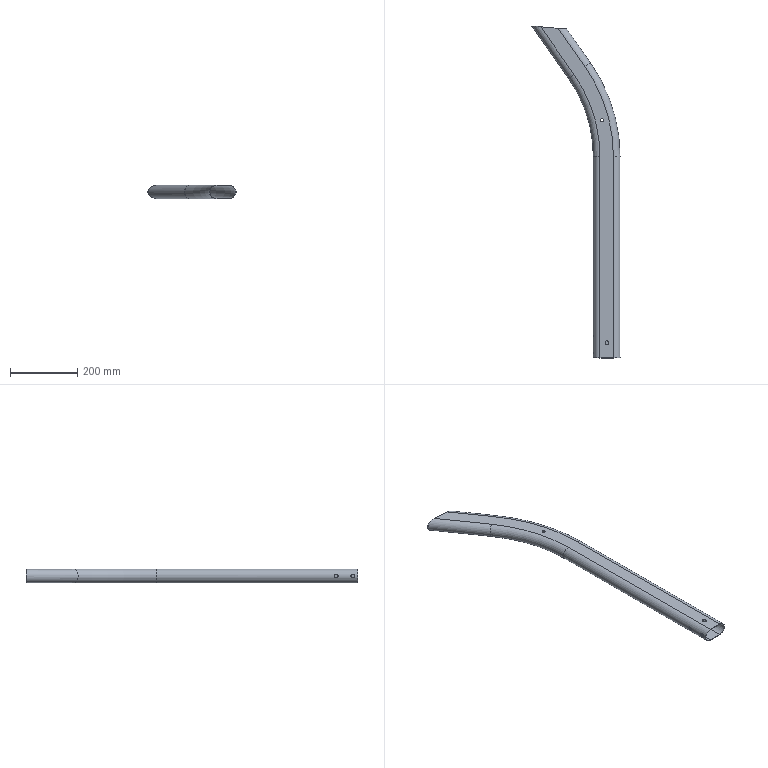Part | STEP file | 6150201L | 1 solid | 34 faces | box 263.127 x 990.805 x 40 mm | volume 310034 mm3 | cylinder 18 | plane 12 | torus 4 | commonest cylinder face diameters 10 x6 9 x4 37 x4 40 x4